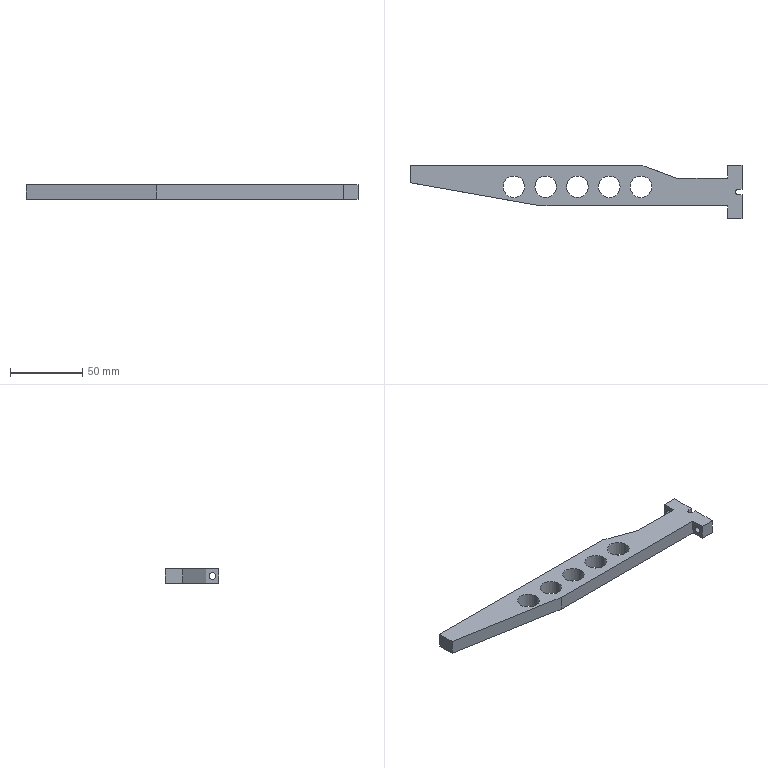Part | 1 solid | 43 faces | box 230 x 37.2 x 10 mm | volume 44801 mm3 | cylinder 21 | plane 16 | cone 6 | commonest cylinder face diameters 15 x10 2.5 x6 4.5 x4 4 x1
STEP:
#1=CARTESIAN_POINT('',(15.5,3.6,0.));
#2=VERTEX_POINT('',#1);
#3=CARTESIAN_POINT('',(30.5,3.6,0.));
#4=VERTEX_POINT('',#3);
#5=CARTESIAN_POINT('',(23.,3.6,0.));
#6=DIRECTION('',(0.,0.,-1.));
#7=DIRECTION('',(-1.,0.,0.));
#8=AXIS2_PLACEMENT_3D('',#5,#6,#7);
#9=CIRCLE('',#8,7.5);
#10=EDGE_CURVE('',#2,#4,#9,.T.);
#11=ORIENTED_EDGE('',*,*,#10,.T.);
#12=CARTESIAN_POINT('',(23.,3.6,0.));
#13=DIRECTION('',(0.,0.,-1.));
#14=DIRECTION('',(-1.,0.,0.));
#15=AXIS2_PLACEMENT_3D('',#12,#13,#14);
#16=CIRCLE('',#15,7.5);
#17=EDGE_CURVE('',#4,#2,#16,.T.);
#18=ORIENTED_EDGE('',*,*,#17,.T.);
#19=EDGE_LOOP('',(#11,#18));
#20=FACE_BOUND('',#19,.T.);
#21=CARTESIAN_POINT('',(37.5,3.6,0.));
#22=VERTEX_POINT('',#21);
#23=CARTESIAN_POINT('',(52.5,3.6,0.));
#24=VERTEX_POINT('',#23);
#25=CARTESIAN_POINT('',(45.,3.6,0.));
#26=DIRECTION('',(0.,0.,-1.));
#27=DIRECTION('',(-1.,0.,0.));
#28=AXIS2_PLACEMENT_3D('',#25,#26,#27);
#29=CIRCLE('',#28,7.5);
#30=EDGE_CURVE('',#22,#24,#29,.T.);
#31=ORIENTED_EDGE('',*,*,#30,.T.);
#32=CARTESIAN_POINT('',(45.,3.6,0.));
#33=DIRECTION('',(0.,0.,-1.));
#34=DIRECTION('',(-1.,0.,0.));
#35=AXIS2_PLACEMENT_3D('',#32,#33,#34);
#36=CIRCLE('',#35,7.5);
#37=EDGE_CURVE('',#24,#22,#36,.T.);
#38=ORIENTED_EDGE('',*,*,#37,.T.);
#39=EDGE_LOOP('',(#31,#38));
#40=FACE_BOUND('',#39,.T.);
#41=CARTESIAN_POINT('',(-50.5,3.6,0.));
#42=VERTEX_POINT('',#41);
#43=CARTESIAN_POINT('',(-35.5,3.6,0.));
#44=VERTEX_POINT('',#43);
#45=CARTESIAN_POINT('',(-43.,3.6,0.));
#46=DIRECTION('',(0.,0.,-1.));
#47=DIRECTION('',(-1.,0.,0.));
#48=AXIS2_PLACEMENT_3D('',#45,#46,#47);
#49=CIRCLE('',#48,7.5);
#50=EDGE_CURVE('',#42,#44,#49,.T.);
#51=ORIENTED_EDGE('',*,*,#50,.T.);
#52=CARTESIAN_POINT('',(-43.,3.6,0.));
#53=DIRECTION('',(0.,0.,-1.));
#54=DIRECTION('',(-1.,0.,0.));
#55=AXIS2_PLACEMENT_3D('',#52,#53,#54);
#56=CIRCLE('',#55,7.5);
#57=EDGE_CURVE('',#44,#42,#56,.T.);
#58=ORIENTED_EDGE('',*,*,#57,.T.);
#59=EDGE_LOOP('',(#51,#58));
#60=FACE_BOUND('',#59,.T.);
#61=CARTESIAN_POINT('',(-28.5,3.6,0.));
#62=VERTEX_POINT('',#61);
#63=CARTESIAN_POINT('',(-13.5,3.6,0.));
#64=VERTEX_POINT('',#63);
#65=CARTESIAN_POINT('',(-21.,3.6,0.));
#66=DIRECTION('',(0.,0.,-1.));
#67=DIRECTION('',(-1.,0.,0.));
#68=AXIS2_PLACEMENT_3D('',#65,#66,#67);
#69=CIRCLE('',#68,7.5);
#70=EDGE_CURVE('',#62,#64,#69,.T.);
#71=ORIENTED_EDGE('',*,*,#70,.T.);
#72=CARTESIAN_POINT('',(-21.,3.6,0.));
#73=DIRECTION('',(0.,0.,-1.));
#74=DIRECTION('',(-1.,0.,0.));
#75=AXIS2_PLACEMENT_3D('',#72,#73,#74);
#76=CIRCLE('',#75,7.5);
#77=EDGE_CURVE('',#64,#62,#76,.T.);
#78=ORIENTED_EDGE('',*,*,#77,.T.);
#79=EDGE_LOOP('',(#71,#78));
#80=FACE_BOUND('',#79,.T.);
#81=CARTESIAN_POINT('',(-6.5,3.6,0.));
#82=VERTEX_POINT('',#81);
#83=CARTESIAN_POINT('',(8.5,3.6,0.));
#84=VERTEX_POINT('',#83);
#85=CARTESIAN_POINT('',(1.,3.6,0.));
#86=DIRECTION('',(0.,0.,-1.));
#87=DIRECTION('',(-1.,0.,0.));
#88=AXIS2_PLACEMENT_3D('',#85,#86,#87);
#89=CIRCLE('',#88,7.5);
#90=EDGE_CURVE('',#82,#84,#89,.T.);
#91=ORIENTED_EDGE('',*,*,#90,.T.);
#92=CARTESIAN_POINT('',(1.,3.6,0.));
#93=DIRECTION('',(0.,0.,-1.));
#94=DIRECTION('',(-1.,0.,0.));
#95=AXIS2_PLACEMENT_3D('',#92,#93,#94);
#96=CIRCLE('',#95,7.5);
#97=EDGE_CURVE('',#84,#82,#96,.T.);
#98=ORIENTED_EDGE('',*,*,#97,.T.);
#99=EDGE_LOOP('',(#91,#98));
#100=FACE_BOUND('',#99,.T.);
#101=CARTESIAN_POINT('',(112.5,2.,0.));
#102=VERTEX_POINT('',#101);
#103=CARTESIAN_POINT('',(112.5,-2.,0.));
#104=VERTEX_POINT('',#103);
#105=CARTESIAN_POINT('',(112.5,0.,0.));
#106=DIRECTION('',(0.,0.,1.));
#107=DIRECTION('',(1.,0.,0.));
#108=AXIS2_PLACEMENT_3D('',#105,#106,#107);
#109=CIRCLE('',#108,2.);
#110=EDGE_CURVE('',#102,#104,#109,.T.);
#111=ORIENTED_EDGE('',*,*,#110,.F.);
#112=CARTESIAN_POINT('',(115.,2.,0.));
#113=VERTEX_POINT('',#112);
#114=CARTESIAN_POINT('',(115.,2.,0.));
#115=DIRECTION('',(1.,0.,0.));
#116=VECTOR('',#115,1000.);
#117=LINE('',#114,#116);
#118=EDGE_CURVE('',#102,#113,#117,.T.);
#119=ORIENTED_EDGE('',*,*,#118,.T.);
#120=CARTESIAN_POINT('',(115.,18.6,0.));
#121=VERTEX_POINT('',#120);
#122=CARTESIAN_POINT('',(115.,18.6,0.));
#123=DIRECTION('',(0.,-1.,0.));
#124=VECTOR('',#123,1000.);
#125=LINE('',#122,#124);
#126=EDGE_CURVE('',#121,#113,#125,.T.);
#127=ORIENTED_EDGE('',*,*,#126,.F.);
#128=CARTESIAN_POINT('',(105.,18.6,0.));
#129=VERTEX_POINT('',#128);
#130=CARTESIAN_POINT('',(115.,18.6,0.));
#131=DIRECTION('',(1.,0.,0.));
#132=VECTOR('',#131,1000.);
#133=LINE('',#130,#132);
#134=EDGE_CURVE('',#129,#121,#133,.T.);
#135=ORIENTED_EDGE('',*,*,#134,.F.);
#136=CARTESIAN_POINT('',(105.,9.6,0.));
#137=VERTEX_POINT('',#136);
#138=CARTESIAN_POINT('',(105.,18.6,0.));
#139=DIRECTION('',(0.,-1.,0.));
#140=VECTOR('',#139,1000.);
#141=LINE('',#138,#140);
#142=EDGE_CURVE('',#129,#137,#141,.T.);
#143=ORIENTED_EDGE('',*,*,#142,.T.);
#144=CARTESIAN_POINT('',(69.727,9.6,0.));
#145=VERTEX_POINT('',#144);
#146=CARTESIAN_POINT('',(105.,9.6,0.));
#147=DIRECTION('',(-1.,0.,0.));
#148=VECTOR('',#147,1000.);
#149=LINE('',#146,#148);
#150=EDGE_CURVE('',#137,#145,#149,.T.);
#151=ORIENTED_EDGE('',*,*,#150,.T.);
#152=CARTESIAN_POINT('',(45.,18.6,0.));
#153=VERTEX_POINT('',#152);
#154=CARTESIAN_POINT('',(69.727,9.6,0.));
#155=DIRECTION('',(-0.9397,0.342,0.));
#156=VECTOR('',#155,1000.);
#157=LINE('',#154,#156);
#158=EDGE_CURVE('',#145,#153,#157,.T.);
#159=ORIENTED_EDGE('',*,*,#158,.T.);
#160=CARTESIAN_POINT('',(-115.,18.6,0.));
#161=VERTEX_POINT('',#160);
#162=CARTESIAN_POINT('',(115.,18.6,0.));
#163=DIRECTION('',(1.,0.,0.));
#164=VECTOR('',#163,1000.);
#165=LINE('',#162,#164);
#166=EDGE_CURVE('',#161,#153,#165,.T.);
#167=ORIENTED_EDGE('',*,*,#166,.F.);
#168=CARTESIAN_POINT('',(-115.,6.4,0.));
#169=VERTEX_POINT('',#168);
#170=CARTESIAN_POINT('',(-115.,18.6,0.));
#171=DIRECTION('',(0.,1.,0.));
#172=VECTOR('',#171,1000.);
#173=LINE('',#170,#172);
#174=EDGE_CURVE('',#169,#161,#173,.T.);
#175=ORIENTED_EDGE('',*,*,#174,.F.);
#176=CARTESIAN_POINT('',(-24.259,-9.6,0.));
#177=VERTEX_POINT('',#176);
#178=CARTESIAN_POINT('',(-24.259,-9.6,0.));
#179=DIRECTION('',(0.9848,-0.1736,0.));
#180=VECTOR('',#179,1000.);
#181=LINE('',#178,#180);
#182=EDGE_CURVE('',#169,#177,#181,.T.);
#183=ORIENTED_EDGE('',*,*,#182,.T.);
#184=CARTESIAN_POINT('',(105.,-9.6,0.));
#185=VERTEX_POINT('',#184);
#186=CARTESIAN_POINT('',(105.,-9.6,0.));
#187=DIRECTION('',(1.,0.,0.));
#188=VECTOR('',#187,1000.);
#189=LINE('',#186,#188);
#190=EDGE_CURVE('',#177,#185,#189,.T.);
#191=ORIENTED_EDGE('',*,*,#190,.T.);
#192=CARTESIAN_POINT('',(105.,-18.6,0.));
#193=VERTEX_POINT('',#192);
#194=CARTESIAN_POINT('',(105.,-18.6,0.));
#195=DIRECTION('',(0.,-1.,0.));
#196=VECTOR('',#195,1000.);
#197=LINE('',#194,#196);
#198=EDGE_CURVE('',#185,#193,#197,.T.);
#199=ORIENTED_EDGE('',*,*,#198,.T.);
#200=CARTESIAN_POINT('',(115.,-18.6,0.));
#201=VERTEX_POINT('',#200);
#202=CARTESIAN_POINT('',(115.,-18.6,0.));
#203=DIRECTION('',(-1.,0.,0.));
#204=VECTOR('',#203,1000.);
#205=LINE('',#202,#204);
#206=EDGE_CURVE('',#201,#193,#205,.T.);
#207=ORIENTED_EDGE('',*,*,#206,.F.);
#208=CARTESIAN_POINT('',(115.,-2.,0.));
#209=VERTEX_POINT('',#208);
#210=CARTESIAN_POINT('',(115.,18.6,0.));
#211=DIRECTION('',(0.,-1.,0.));
#212=VECTOR('',#211,1000.);
#213=LINE('',#210,#212);
#214=EDGE_CURVE('',#209,#201,#213,.T.);
#215=ORIENTED_EDGE('',*,*,#214,.F.);
#216=CARTESIAN_POINT('',(115.,-2.,0.));
#217=DIRECTION('',(-1.,0.,0.));
#218=VECTOR('',#217,1000.);
#219=LINE('',#216,#218);
#220=EDGE_CURVE('',#209,#104,#219,.T.);
#221=ORIENTED_EDGE('',*,*,#220,.T.);
#222=EDGE_LOOP('',(#111,#119,#127,#135,#143,#151,#159,#167,#175,#183,#191,#199,#207,#215,#221));
#223=FACE_BOUND('',#222,.T.);
#224=CARTESIAN_POINT('',(0.,0.,0.));
#225=DIRECTION('',(0.,0.,-1.));
#226=DIRECTION('',(1.,0.,0.));
#227=AXIS2_PLACEMENT_3D('',#224,#225,#226);
#228=PLANE('',#227);
#229=ADVANCED_FACE('',(#20,#40,#60,#80,#100,#223),#228,.F.);
#230=CARTESIAN_POINT('',(115.,-16.35,-5.));
#231=VERTEX_POINT('',#230);
#232=CARTESIAN_POINT('',(115.,-11.85,-5.));
#233=VERTEX_POINT('',#232);
#234=CARTESIAN_POINT('',(115.,-14.1,-5.));
#235=DIRECTION('',(-1.,0.,0.));
#236=DIRECTION('',(0.,-1.,0.));
#237=AXIS2_PLACEMENT_3D('',#234,#235,#236);
#238=CIRCLE('',#237,2.25);
#239=EDGE_CURVE('',#231,#233,#238,.T.);
#240=ORIENTED_EDGE('',*,*,#239,.F.);
#241=CARTESIAN_POINT('',(105.,-16.35,-5.));
#242=VERTEX_POINT('',#241);
#243=CARTESIAN_POINT('',(115.,-16.35,-5.));
#244=DIRECTION('',(-1.,0.,0.));
#245=VECTOR('',#244,1000.);
#246=LINE('',#243,#245);
#247=EDGE_CURVE('',#231,#242,#246,.T.);
#248=ORIENTED_EDGE('',*,*,#247,.T.);
#249=CARTESIAN_POINT('',(105.,-11.85,-5.));
#250=VERTEX_POINT('',#249);
#251=CARTESIAN_POINT('',(105.,-14.1,-5.));
#252=DIRECTION('',(-1.,0.,0.));
#253=DIRECTION('',(0.,-1.,0.));
#254=AXIS2_PLACEMENT_3D('',#251,#252,#253);
#255=CIRCLE('',#254,2.25);
#256=EDGE_CURVE('',#242,#250,#255,.T.);
#257=ORIENTED_EDGE('',*,*,#256,.T.);
#258=CARTESIAN_POINT('',(115.,-11.85,-5.));
#259=DIRECTION('',(-1.,0.,0.));
#260=VECTOR('',#259,1000.);
#261=LINE('',#258,#260);
#262=EDGE_CURVE('',#233,#250,#261,.T.);
#263=ORIENTED_EDGE('',*,*,#262,.F.);
#264=EDGE_LOOP('',(#240,#248,#257,#263));
#265=FACE_BOUND('',#264,.T.);
#266=CARTESIAN_POINT('',(115.,-14.1,-5.));
#267=DIRECTION('',(-1.,0.,0.));
#268=DIRECTION('',(0.,-1.,0.));
#269=AXIS2_PLACEMENT_3D('',#266,#267,#268);
#270=CYLINDRICAL_SURFACE('',#269,2.25);
#271=ADVANCED_FACE('',(#265),#270,.F.);
#272=CARTESIAN_POINT('',(115.,11.85,-5.));
#273=VERTEX_POINT('',#272);
#274=CARTESIAN_POINT('',(115.,16.35,-5.));
#275=VERTEX_POINT('',#274);
#276=CARTESIAN_POINT('',(115.,14.1,-5.));
#277=DIRECTION('',(-1.,0.,0.));
#278=DIRECTION('',(0.,1.,0.));
#279=AXIS2_PLACEMENT_3D('',#276,#277,#278);
#280=CIRCLE('',#279,2.25);
#281=EDGE_CURVE('',#273,#275,#280,.T.);
#282=ORIENTED_EDGE('',*,*,#281,.F.);
#283=CARTESIAN_POINT('',(105.,11.85,-5.));
#284=VERTEX_POINT('',#283);
#285=CARTESIAN_POINT('',(115.,11.85,-5.));
#286=DIRECTION('',(-1.,0.,0.));
#287=VECTOR('',#286,1000.);
#288=LINE('',#285,#287);
#289=EDGE_CURVE('',#273,#284,#288,.T.);
#290=ORIENTED_EDGE('',*,*,#289,.T.);
#291=CARTESIAN_POINT('',(105.,16.35,-5.));
#292=VERTEX_POINT('',#291);
#293=CARTESIAN_POINT('',(105.,14.1,-5.));
#294=DIRECTION('',(-1.,0.,0.));
#295=DIRECTION('',(0.,1.,0.));
#296=AXIS2_PLACEMENT_3D('',#293,#294,#295);
#297=CIRCLE('',#296,2.25);
#298=EDGE_CURVE('',#284,#292,#297,.T.);
#299=ORIENTED_EDGE('',*,*,#298,.T.);
#300=CARTESIAN_POINT('',(115.,16.35,-5.));
#301=DIRECTION('',(-1.,0.,0.));
#302=VECTOR('',#301,1000.);
#303=LINE('',#300,#302);
#304=EDGE_CURVE('',#275,#292,#303,.T.);
#305=ORIENTED_EDGE('',*,*,#304,.F.);
#306=EDGE_LOOP('',(#282,#290,#299,#305));
#307=FACE_BOUND('',#306,.T.);
#308=CARTESIAN_POINT('',(115.,14.1,-5.));
#309=DIRECTION('',(-1.,0.,0.));
#310=DIRECTION('',(0.,-1.,0.));
#311=AXIS2_PLACEMENT_3D('',#308,#309,#310);
#312=CYLINDRICAL_SURFACE('',#311,2.25);
#313=ADVANCED_FACE('',(#307),#312,.F.);
#314=CARTESIAN_POINT('',(55.,11.1,-6.25));
#315=VERTEX_POINT('',#314);
#316=CARTESIAN_POINT('',(55.,10.349,-5.));
#317=VERTEX_POINT('',#316);
#318=CARTESIAN_POINT('',(55.,11.1,-6.25));
#319=DIRECTION('',(0.,0.515,-0.8572));
#320=VECTOR('',#319,1000.);
#321=LINE('',#318,#320);
#322=EDGE_CURVE('',#315,#317,#321,.F.);
#323=ORIENTED_EDGE('',*,*,#322,.T.);
#324=CARTESIAN_POINT('',(55.,11.1,-3.75));
#325=VERTEX_POINT('',#324);
#326=CARTESIAN_POINT('',(55.,11.1,-3.75));
#327=DIRECTION('',(0.,0.515,0.8572));
#328=VECTOR('',#327,1000.);
#329=LINE('',#326,#328);
#330=EDGE_CURVE('',#325,#317,#329,.F.);
#331=ORIENTED_EDGE('',*,*,#330,.F.);
#332=CARTESIAN_POINT('',(55.,11.1,-5.));
#333=DIRECTION('',(0.,1.,0.));
#334=DIRECTION('',(0.,0.,-1.));
#335=AXIS2_PLACEMENT_3D('',#332,#333,#334);
#336=CIRCLE('',#335,1.25);
#337=EDGE_CURVE('',#325,#315,#336,.T.);
#338=ORIENTED_EDGE('',*,*,#337,.T.);
#339=EDGE_LOOP('',(#323,#331,#338));
#340=FACE_BOUND('',#339,.T.);
#341=CARTESIAN_POINT('',(55.,11.1,-5.));
#342=DIRECTION('',(0.,1.,0.));
#343=DIRECTION('',(0.,0.,1.));
#344=AXIS2_PLACEMENT_3D('',#341,#342,#343);
#345=CONICAL_SURFACE('',#344,1.25,1.03);
#346=ADVANCED_FACE('',(#340),#345,.F.);
#347=ORIENTED_EDGE('',*,*,#337,.F.);
#348=CARTESIAN_POINT('',(55.,14.96,-3.75));
#349=VERTEX_POINT('',#348);
#350=CARTESIAN_POINT('',(55.,18.6,-3.75));
#351=DIRECTION('',(0.,1.,0.));
#352=VECTOR('',#351,1000.);
#353=LINE('',#350,#352);
#354=EDGE_CURVE('',#349,#325,#353,.F.);
#355=ORIENTED_EDGE('',*,*,#354,.F.);
#356=CARTESIAN_POINT('',(55.,14.96,-6.25));
#357=VERTEX_POINT('',#356);
#358=CARTESIAN_POINT('',(55.,14.96,-6.25));
#359=CARTESIAN_POINT('',(57.5,14.05,-6.25));
#360=CARTESIAN_POINT('',(57.5,14.05,-3.75));
#361=CARTESIAN_POINT('',(55.,14.96,-3.75));
#362=(BOUNDED_CURVE()B_SPLINE_CURVE(3,(#358,#359,#360,#361),.UNSPECIFIED.,.F.,.F.)B_SPLINE_CURVE_WITH_KNOTS((4,4),(0.,1.),.PIECEWISE_BEZIER_KNOTS.)CURVE()GEOMETRIC_REPRESENTATION_ITEM()RATIONAL_B_SPLINE_CURVE((1.,0.3333,0.3333,1.))REPRESENTATION_ITEM(''));
#363=EDGE_CURVE('',#357,#349,#362,.T.);
#364=ORIENTED_EDGE('',*,*,#363,.F.);
#365=CARTESIAN_POINT('',(55.,18.6,-6.25));
#366=DIRECTION('',(0.,1.,0.));
#367=VECTOR('',#366,1000.);
#368=LINE('',#365,#367);
#369=EDGE_CURVE('',#357,#315,#368,.F.);
#370=ORIENTED_EDGE('',*,*,#369,.T.);
#371=EDGE_LOOP('',(#347,#355,#364,#370));
#372=FACE_BOUND('',#371,.T.);
#373=CARTESIAN_POINT('',(55.,18.6,-5.));
#374=DIRECTION('',(0.,1.,0.));
#375=DIRECTION('',(0.,0.,1.));
#376=AXIS2_PLACEMENT_3D('',#373,#374,#375);
#377=CYLINDRICAL_SURFACE('',#376,1.25);
#378=ADVANCED_FACE('',(#372),#377,.F.);
#379=CARTESIAN_POINT('',(-25.,11.1,-3.75));
#380=VERTEX_POINT('',#379);
#381=CARTESIAN_POINT('',(-25.,11.1,-6.25));
#382=VERTEX_POINT('',#381);
#383=CARTESIAN_POINT('',(-25.,11.1,-5.));
#384=DIRECTION('',(0.,1.,0.));
#385=DIRECTION('',(0.,0.,-1.));
#386=AXIS2_PLACEMENT_3D('',#383,#384,#385);
#387=CIRCLE('',#386,1.25);
#388=EDGE_CURVE('',#380,#382,#387,.T.);
#389=ORIENTED_EDGE('',*,*,#388,.F.);
#390=CARTESIAN_POINT('',(-25.,18.6,-3.75));
#391=VERTEX_POINT('',#390);
#392=CARTESIAN_POINT('',(-25.,18.6,-3.75));
#393=DIRECTION('',(0.,1.,0.));
#394=VECTOR('',#393,1000.);
#395=LINE('',#392,#394);
#396=EDGE_CURVE('',#391,#380,#395,.F.);
#397=ORIENTED_EDGE('',*,*,#396,.F.);
#398=CARTESIAN_POINT('',(-25.,18.6,-6.25));
#399=VERTEX_POINT('',#398);
#400=CARTESIAN_POINT('',(-25.,18.6,-5.));
#401=DIRECTION('',(0.,1.,0.));
#402=DIRECTION('',(0.,0.,-1.));
#403=AXIS2_PLACEMENT_3D('',#400,#401,#402);
#404=CIRCLE('',#403,1.25);
#405=EDGE_CURVE('',#391,#399,#404,.T.);
#406=ORIENTED_EDGE('',*,*,#405,.T.);
#407=CARTESIAN_POINT('',(-25.,18.6,-6.25));
#408=DIRECTION('',(0.,1.,0.));
#409=VECTOR('',#408,1000.);
#410=LINE('',#407,#409);
#411=EDGE_CURVE('',#399,#382,#410,.F.);
#412=ORIENTED_EDGE('',*,*,#411,.T.);
#413=EDGE_LOOP('',(#389,#397,#406,#412));
#414=FACE_BOUND('',#413,.T.);
#415=CARTESIAN_POINT('',(-25.,18.6,-5.));
#416=DIRECTION('',(0.,1.,0.));
#417=DIRECTION('',(0.,0.,1.));
#418=AXIS2_PLACEMENT_3D('',#415,#416,#417);
#419=CYLINDRICAL_SURFACE('',#418,1.25);
#420=ADVANCED_FACE('',(#414),#419,.F.);
#421=CARTESIAN_POINT('',(-25.,10.349,-5.));
#422=VERTEX_POINT('',#421);
#423=CARTESIAN_POINT('',(-25.,11.1,-6.25));
#424=DIRECTION('',(0.,0.515,-0.8572));
#425=VECTOR('',#424,1000.);
#426=LINE('',#423,#425);
#427=EDGE_CURVE('',#382,#422,#426,.F.);
#428=ORIENTED_EDGE('',*,*,#427,.T.);
#429=CARTESIAN_POINT('',(-25.,11.1,-3.75));
#430=DIRECTION('',(0.,0.515,0.8572));
#431=VECTOR('',#430,1000.);
#432=LINE('',#429,#431);
#433=EDGE_CURVE('',#380,#422,#432,.F.);
#434=ORIENTED_EDGE('',*,*,#433,.F.);
#435=ORIENTED_EDGE('',*,*,#388,.T.);
#436=EDGE_LOOP('',(#428,#434,#435));
#437=FACE_BOUND('',#436,.T.);
#438=CARTESIAN_POINT('',(-25.,11.1,-5.));
#439=DIRECTION('',(0.,1.,0.));
#440=DIRECTION('',(0.,0.,1.));
#441=AXIS2_PLACEMENT_3D('',#438,#439,#440);
#442=CONICAL_SURFACE('',#441,1.25,1.03);
#443=ADVANCED_FACE('',(#437),#442,.F.);
#444=CARTESIAN_POINT('',(-105.,11.1,-3.75));
#445=VERTEX_POINT('',#444);
#446=CARTESIAN_POINT('',(-105.,11.1,-6.25));
#447=VERTEX_POINT('',#446);
#448=CARTESIAN_POINT('',(-105.,11.1,-5.));
#449=DIRECTION('',(0.,1.,0.));
#450=DIRECTION('',(0.,0.,-1.));
#451=AXIS2_PLACEMENT_3D('',#448,#449,#450);
#452=CIRCLE('',#451,1.25);
#453=EDGE_CURVE('',#445,#447,#452,.T.);
#454=ORIENTED_EDGE('',*,*,#453,.F.);
#455=CARTESIAN_POINT('',(-105.,18.6,-3.75));
#456=VERTEX_POINT('',#455);
#457=CARTESIAN_POINT('',(-105.,18.6,-3.75));
#458=DIRECTION('',(0.,1.,0.));
#459=VECTOR('',#458,1000.);
#460=LINE('',#457,#459);
#461=EDGE_CURVE('',#456,#445,#460,.F.);
#462=ORIENTED_EDGE('',*,*,#461,.F.);
#463=CARTESIAN_POINT('',(-105.,18.6,-6.25));
#464=VERTEX_POINT('',#463);
#465=CARTESIAN_POINT('',(-105.,18.6,-5.));
#466=DIRECTION('',(0.,1.,0.));
#467=DIRECTION('',(0.,0.,-1.));
#468=AXIS2_PLACEMENT_3D('',#465,#466,#467);
#469=CIRCLE('',#468,1.25);
#470=EDGE_CURVE('',#456,#464,#469,.T.);
#471=ORIENTED_EDGE('',*,*,#470,.T.);
#472=CARTESIAN_POINT('',(-105.,18.6,-6.25));
#473=DIRECTION('',(0.,1.,0.));
#474=VECTOR('',#473,1000.);
#475=LINE('',#472,#474);
#476=EDGE_CURVE('',#464,#447,#475,.F.);
#477=ORIENTED_EDGE('',*,*,#476,.T.);
#478=EDGE_LOOP('',(#454,#462,#471,#477));
#479=FACE_BOUND('',#478,.T.);
#480=CARTESIAN_POINT('',(-105.,18.6,-5.));
#481=DIRECTION('',(0.,1.,0.));
#482=DIRECTION('',(0.,0.,1.));
#483=AXIS2_PLACEMENT_3D('',#480,#481,#482);
#484=CYLINDRICAL_SURFACE('',#483,1.25);
#485=ADVANCED_FACE('',(#479),#484,.F.);
#486=CARTESIAN_POINT('',(-105.,10.349,-5.));
#487=VERTEX_POINT('',#486);
#488=CARTESIAN_POINT('',(-105.,11.1,-6.25));
#489=DIRECTION('',(0.,0.515,-0.8572));
#490=VECTOR('',#489,1000.);
#491=LINE('',#488,#490);
#492=EDGE_CURVE('',#447,#487,#491,.F.);
#493=ORIENTED_EDGE('',*,*,#492,.T.);
#494=CARTESIAN_POINT('',(-105.,11.1,-3.75));
#495=DIRECTION('',(0.,0.515,0.8572));
#496=VECTOR('',#495,1000.);
#497=LINE('',#494,#496);
#498=EDGE_CURVE('',#445,#487,#497,.F.);
#499=ORIENTED_EDGE('',*,*,#498,.F.);
#500=ORIENTED_EDGE('',*,*,#453,.T.);
#501=EDGE_LOOP('',(#493,#499,#500));
#502=FACE_BOUND('',#501,.T.);
#503=CARTESIAN_POINT('',(-105.,11.1,-5.));
#504=DIRECTION('',(0.,1.,0.));
#505=DIRECTION('',(0.,0.,1.));
#506=AXIS2_PLACEMENT_3D('',#503,#504,#505);
#507=CONICAL_SURFACE('',#506,1.25,1.03);
#508=ADVANCED_FACE('',(#502),#507,.F.);
#509=ORIENTED_EDGE('',*,*,#97,.F.);
#510=CARTESIAN_POINT('',(8.5,3.6,-10.));
#511=VERTEX_POINT('',#510);
#512=CARTESIAN_POINT('',(8.5,3.6,0.));
#513=DIRECTION('',(0.,0.,-1.));
#514=VECTOR('',#513,1000.);
#515=LINE('',#512,#514);
#516=EDGE_CURVE('',#511,#84,#515,.F.);
#517=ORIENTED_EDGE('',*,*,#516,.F.);
#518=CARTESIAN_POINT('',(-6.5,3.6,-10.));
#519=VERTEX_POINT('',#518);
#520=CARTESIAN_POINT('',(1.,3.6,-10.));
#521=DIRECTION('',(0.,0.,-1.));
#522=DIRECTION('',(-1.,0.,0.));
#523=AXIS2_PLACEMENT_3D('',#520,#521,#522);
#524=CIRCLE('',#523,7.5);
#525=EDGE_CURVE('',#511,#519,#524,.T.);
#526=ORIENTED_EDGE('',*,*,#525,.T.);
#527=CARTESIAN_POINT('',(-6.5,3.6,0.));
#528=DIRECTION('',(0.,0.,-1.));
#529=VECTOR('',#528,1000.);
#530=LINE('',#527,#529);
#531=EDGE_CURVE('',#519,#82,#530,.F.);
#532=ORIENTED_EDGE('',*,*,#531,.T.);
#533=EDGE_LOOP('',(#509,#517,#526,#532));
#534=FACE_BOUND('',#533,.T.);
#535=CARTESIAN_POINT('',(1.,3.6,0.));
#536=DIRECTION('',(0.,0.,-1.));
#537=DIRECTION('',(1.,0.,0.));
#538=AXIS2_PLACEMENT_3D('',#535,#536,#537);
#539=CYLINDRICAL_SURFACE('',#538,7.5);
#540=ADVANCED_FACE('',(#534),#539,.F.);
#541=ORIENTED_EDGE('',*,*,#77,.F.);
#542=CARTESIAN_POINT('',(-13.5,3.6,-10.));
#543=VERTEX_POINT('',#542);
#544=CARTESIAN_POINT('',(-13.5,3.6,0.));
#545=DIRECTION('',(0.,0.,-1.));
#546=VECTOR('',#545,1000.);
#547=LINE('',#544,#546);
#548=EDGE_CURVE('',#543,#64,#547,.F.);
#549=ORIENTED_EDGE('',*,*,#548,.F.);
#550=CARTESIAN_POINT('',(-28.5,3.6,-10.));
#551=VERTEX_POINT('',#550);
#552=CARTESIAN_POINT('',(-21.,3.6,-10.));
#553=DIRECTION('',(0.,0.,-1.));
#554=DIRECTION('',(-1.,0.,0.));
#555=AXIS2_PLACEMENT_3D('',#552,#553,#554);
#556=CIRCLE('',#555,7.5);
#557=EDGE_CURVE('',#543,#551,#556,.T.);
#558=ORIENTED_EDGE('',*,*,#557,.T.);
#559=CARTESIAN_POINT('',(-28.5,3.6,0.));
#560=DIRECTION('',(0.,0.,-1.));
#561=VECTOR('',#560,1000.);
#562=LINE('',#559,#561);
#563=EDGE_CURVE('',#551,#62,#562,.F.);
#564=ORIENTED_EDGE('',*,*,#563,.T.);
#565=EDGE_LOOP('',(#541,#549,#558,#564));
#566=FACE_BOUND('',#565,.T.);
#567=CARTESIAN_POINT('',(-21.,3.6,0.));
#568=DIRECTION('',(0.,0.,-1.));
#569=DIRECTION('',(1.,0.,0.));
#570=AXIS2_PLACEMENT_3D('',#567,#568,#569);
#571=CYLINDRICAL_SURFACE('',#570,7.5);
#572=ADVANCED_FACE('',(#566),#571,.F.);
#573=ORIENTED_EDGE('',*,*,#57,.F.);
#574=CARTESIAN_POINT('',(-35.5,3.6,-10.));
#575=VERTEX_POINT('',#574);
#576=CARTESIAN_POINT('',(-35.5,3.6,0.));
#577=DIRECTION('',(0.,0.,-1.));
#578=VECTOR('',#577,1000.);
#579=LINE('',#576,#578);
#580=EDGE_CURVE('',#575,#44,#579,.F.);
#581=ORIENTED_EDGE('',*,*,#580,.F.);
#582=CARTESIAN_POINT('',(-50.5,3.6,-10.));
#583=VERTEX_POINT('',#582);
#584=CARTESIAN_POINT('',(-43.,3.6,-10.));
#585=DIRECTION('',(0.,0.,-1.));
#586=DIRECTION('',(-1.,0.,0.));
#587=AXIS2_PLACEMENT_3D('',#584,#585,#586);
#588=CIRCLE('',#587,7.5);
#589=EDGE_CURVE('',#575,#583,#588,.T.);
#590=ORIENTED_EDGE('',*,*,#589,.T.);
#591=CARTESIAN_POINT('',(-50.5,3.6,0.));
#592=DIRECTION('',(0.,0.,-1.));
#593=VECTOR('',#592,1000.);
#594=LINE('',#591,#593);
#595=EDGE_CURVE('',#583,#42,#594,.F.);
#596=ORIENTED_EDGE('',*,*,#595,.T.);
#597=EDGE_LOOP('',(#573,#581,#590,#596));
#598=FACE_BOUND('',#597,.T.);
#599=CARTESIAN_POINT('',(-43.,3.6,0.));
#600=DIRECTION('',(0.,0.,-1.));
#601=DIRECTION('',(1.,0.,0.));
#602=AXIS2_PLACEMENT_3D('',#599,#600,#601);
#603=CYLINDRICAL_SURFACE('',#602,7.5);
#604=ADVANCED_FACE('',(#598),#603,.F.);
#605=ORIENTED_EDGE('',*,*,#37,.F.);
#606=CARTESIAN_POINT('',(52.5,3.6,-10.));
#607=VERTEX_POINT('',#606);
#608=CARTESIAN_POINT('',(52.5,3.6,0.));
#609=DIRECTION('',(0.,0.,-1.));
#610=VECTOR('',#609,1000.);
#611=LINE('',#608,#610);
#612=EDGE_CURVE('',#607,#24,#611,.F.);
#613=ORIENTED_EDGE('',*,*,#612,.F.);
#614=CARTESIAN_POINT('',(37.5,3.6,-10.));
#615=VERTEX_POINT('',#614);
#616=CARTESIAN_POINT('',(45.,3.6,-10.));
#617=DIRECTION('',(0.,0.,-1.));
#618=DIRECTION('',(-1.,0.,0.));
#619=AXIS2_PLACEMENT_3D('',#616,#617,#618);
#620=CIRCLE('',#619,7.5);
#621=EDGE_CURVE('',#607,#615,#620,.T.);
#622=ORIENTED_EDGE('',*,*,#621,.T.);
#623=CARTESIAN_POINT('',(37.5,3.6,0.));
#624=DIRECTION('',(0.,0.,-1.));
#625=VECTOR('',#624,1000.);
#626=LINE('',#623,#625);
#627=EDGE_CURVE('',#615,#22,#626,.F.);
#628=ORIENTED_EDGE('',*,*,#627,.T.);
#629=EDGE_LOOP('',(#605,#613,#622,#628));
#630=FACE_BOUND('',#629,.T.);
#631=CARTESIAN_POINT('',(45.,3.6,0.));
#632=DIRECTION('',(0.,0.,-1.));
#633=DIRECTION('',(1.,0.,0.));
#634=AXIS2_PLACEMENT_3D('',#631,#632,#633);
#635=CYLINDRICAL_SURFACE('',#634,7.5);
#636=ADVANCED_FACE('',(#630),#635,.F.);
#637=ORIENTED_EDGE('',*,*,#17,.F.);
#638=CARTESIAN_POINT('',(30.5,3.6,-10.));
#639=VERTEX_POINT('',#638);
#640=CARTESIAN_POINT('',(30.5,3.6,0.));
#641=DIRECTION('',(0.,0.,-1.));
#642=VECTOR('',#641,1000.);
#643=LINE('',#640,#642);
#644=EDGE_CURVE('',#639,#4,#643,.F.);
#645=ORIENTED_EDGE('',*,*,#644,.F.);
#646=CARTESIAN_POINT('',(15.5,3.6,-10.));
#647=VERTEX_POINT('',#646);
#648=CARTESIAN_POINT('',(23.,3.6,-10.));
#649=DIRECTION('',(0.,0.,-1.));
#650=DIRECTION('',(-1.,0.,0.));
#651=AXIS2_PLACEMENT_3D('',#648,#649,#650);
#652=CIRCLE('',#651,7.5);
#653=EDGE_CURVE('',#639,#647,#652,.T.);
#654=ORIENTED_EDGE('',*,*,#653,.T.);
#655=CARTESIAN_POINT('',(15.5,3.6,0.));
#656=DIRECTION('',(0.,0.,-1.));
#657=VECTOR('',#656,1000.);
#658=LINE('',#655,#657);
#659=EDGE_CURVE('',#647,#2,#658,.F.);
#660=ORIENTED_EDGE('',*,*,#659,.T.);
#661=EDGE_LOOP('',(#637,#645,#654,#660));
#662=FACE_BOUND('',#661,.T.);
#663=CARTESIAN_POINT('',(23.,3.6,0.));
#664=DIRECTION('',(0.,0.,-1.));
#665=DIRECTION('',(1.,0.,0.));
#666=AXIS2_PLACEMENT_3D('',#663,#664,#665);
#667=CYLINDRICAL_SURFACE('',#666,7.5);
#668=ADVANCED_FACE('',(#662),#667,.F.);
#669=CARTESIAN_POINT('',(115.,14.1,-5.));
#670=DIRECTION('',(-1.,0.,0.));
#671=DIRECTION('',(0.,1.,0.));
#672=AXIS2_PLACEMENT_3D('',#669,#670,#671);
#673=CIRCLE('',#672,2.25);
#674=EDGE_CURVE('',#275,#273,#673,.T.);
#675=ORIENTED_EDGE('',*,*,#674,.T.);
#676=ORIENTED_EDGE('',*,*,#281,.T.);
#677=EDGE_LOOP('',(#675,#676));
#678=FACE_BOUND('',#677,.T.);
#679=ORIENTED_EDGE('',*,*,#126,.T.);
#680=CARTESIAN_POINT('',(115.,2.,-10.));
#681=VERTEX_POINT('',#680);
#682=CARTESIAN_POINT('',(115.,2.,0.));
#683=DIRECTION('',(0.,0.,-1.));
#684=VECTOR('',#683,1000.);
#685=LINE('',#682,#684);
#686=EDGE_CURVE('',#113,#681,#685,.T.);
#687=ORIENTED_EDGE('',*,*,#686,.T.);
#688=CARTESIAN_POINT('',(115.,18.6,-10.));
#689=VERTEX_POINT('',#688);
#690=CARTESIAN_POINT('',(115.,18.6,-10.));
#691=DIRECTION('',(0.,-1.,0.));
#692=VECTOR('',#691,1000.);
#693=LINE('',#690,#692);
#694=EDGE_CURVE('',#689,#681,#693,.T.);
#695=ORIENTED_EDGE('',*,*,#694,.F.);
#696=CARTESIAN_POINT('',(115.,18.6,-10.));
#697=DIRECTION('',(0.,0.,1.));
#698=VECTOR('',#697,1000.);
#699=LINE('',#696,#698);
#700=EDGE_CURVE('',#689,#121,#699,.T.);
#701=ORIENTED_EDGE('',*,*,#700,.T.);
#702=EDGE_LOOP('',(#679,#687,#695,#701));
#703=FACE_BOUND('',#702,.T.);
#704=CARTESIAN_POINT('',(115.,18.6,-10.));
#705=DIRECTION('',(-1.,0.,0.));
#706=DIRECTION('',(0.,0.,-1.));
#707=AXIS2_PLACEMENT_3D('',#704,#705,#706);
#708=PLANE('',#707);
#709=ADVANCED_FACE('',(#678,#703),#708,.F.);
#710=CARTESIAN_POINT('',(-25.,18.6,-5.));
#711=DIRECTION('',(0.,1.,0.));
#712=DIRECTION('',(0.,0.,-1.));
#713=AXIS2_PLACEMENT_3D('',#710,#711,#712);
#714=CIRCLE('',#713,1.25);
#715=EDGE_CURVE('',#399,#391,#714,.T.);
#716=ORIENTED_EDGE('',*,*,#715,.F.);
#717=ORIENTED_EDGE('',*,*,#405,.F.);
#718=EDGE_LOOP('',(#716,#717));
#719=FACE_BOUND('',#718,.T.);
#720=CARTESIAN_POINT('',(-105.,18.6,-5.));
#721=DIRECTION('',(0.,1.,0.));
#722=DIRECTION('',(0.,0.,-1.));
#723=AXIS2_PLACEMENT_3D('',#720,#721,#722);
#724=CIRCLE('',#723,1.25);
#725=EDGE_CURVE('',#464,#456,#724,.T.);
#726=ORIENTED_EDGE('',*,*,#725,.F.);
#727=ORIENTED_EDGE('',*,*,#470,.F.);
#728=EDGE_LOOP('',(#726,#727));
#729=FACE_BOUND('',#728,.T.);
#730=ORIENTED_EDGE('',*,*,#166,.T.);
#731=CARTESIAN_POINT('',(45.,18.6,-10.));
#732=VERTEX_POINT('',#731);
#733=CARTESIAN_POINT('',(45.,18.6,0.));
#734=DIRECTION('',(0.,0.,-1.));
#735=VECTOR('',#734,1000.);
#736=LINE('',#733,#735);
#737=EDGE_CURVE('',#153,#732,#736,.T.);
#738=ORIENTED_EDGE('',*,*,#737,.T.);
#739=CARTESIAN_POINT('',(-115.,18.6,-10.));
#740=VERTEX_POINT('',#739);
#741=CARTESIAN_POINT('',(115.,18.6,-10.));
#742=DIRECTION('',(1.,0.,0.));
#743=VECTOR('',#742,1000.);
#744=LINE('',#741,#743);
#745=EDGE_CURVE('',#740,#732,#744,.T.);
#746=ORIENTED_EDGE('',*,*,#745,.F.);
#747=CARTESIAN_POINT('',(-115.,18.6,-10.));
#748=DIRECTION('',(0.,0.,1.));
#749=VECTOR('',#748,1000.);
#750=LINE('',#747,#749);
#751=EDGE_CURVE('',#740,#161,#750,.T.);
#752=ORIENTED_EDGE('',*,*,#751,.T.);
#753=EDGE_LOOP('',(#730,#738,#746,#752));
#754=FACE_BOUND('',#753,.T.);
#755=CARTESIAN_POINT('',(115.,18.6,-10.));
#756=DIRECTION('',(0.,-1.,0.));
#757=DIRECTION('',(0.,0.,-1.));
#758=AXIS2_PLACEMENT_3D('',#755,#756,#757);
#759=PLANE('',#758);
#760=ADVANCED_FACE('',(#719,#729,#754),#759,.F.);
#761=CARTESIAN_POINT('',(115.,-14.1,-5.));
#762=DIRECTION('',(-1.,0.,0.));
#763=DIRECTION('',(0.,-1.,0.));
#764=AXIS2_PLACEMENT_3D('',#761,#762,#763);
#765=CIRCLE('',#764,2.25);
#766=EDGE_CURVE('',#233,#231,#765,.T.);
#767=ORIENTED_EDGE('',*,*,#766,.T.);
#768=ORIENTED_EDGE('',*,*,#239,.T.);
#769=EDGE_LOOP('',(#767,#768));
#770=FACE_BOUND('',#769,.T.);
#771=CARTESIAN_POINT('',(115.,-2.,-10.));
#772=VERTEX_POINT('',#771);
#773=CARTESIAN_POINT('',(115.,-18.6,-10.));
#774=VERTEX_POINT('',#773);
#775=CARTESIAN_POINT('',(115.,18.6,-10.));
#776=DIRECTION('',(0.,-1.,0.));
#777=VECTOR('',#776,1000.);
#778=LINE('',#775,#777);
#779=EDGE_CURVE('',#772,#774,#778,.T.);
#780=ORIENTED_EDGE('',*,*,#779,.F.);
#781=CARTESIAN_POINT('',(115.,-2.,0.));
#782=DIRECTION('',(0.,0.,-1.));
#783=VECTOR('',#782,1000.);
#784=LINE('',#781,#783);
#785=EDGE_CURVE('',#209,#772,#784,.T.);
#786=ORIENTED_EDGE('',*,*,#785,.F.);
#787=ORIENTED_EDGE('',*,*,#214,.T.);
#788=CARTESIAN_POINT('',(115.,-18.6,-10.));
#789=DIRECTION('',(0.,0.,1.));
#790=VECTOR('',#789,1000.);
#791=LINE('',#788,#790);
#792=EDGE_CURVE('',#774,#201,#791,.T.);
#793=ORIENTED_EDGE('',*,*,#792,.F.);
#794=EDGE_LOOP('',(#780,#786,#787,#793));
#795=FACE_BOUND('',#794,.T.);
#796=CARTESIAN_POINT('',(115.,18.6,-10.));
#797=DIRECTION('',(-1.,0.,0.));
#798=DIRECTION('',(0.,0.,-1.));
#799=AXIS2_PLACEMENT_3D('',#796,#797,#798);
#800=PLANE('',#799);
#801=ADVANCED_FACE('',(#770,#795),#800,.F.);
#802=ORIENTED_EDGE('',*,*,#206,.T.);
#803=CARTESIAN_POINT('',(105.,-18.6,-10.));
#804=VERTEX_POINT('',#803);
#805=CARTESIAN_POINT('',(105.,-18.6,0.));
#806=DIRECTION('',(0.,0.,-1.));
#807=VECTOR('',#806,1000.);
#808=LINE('',#805,#807);
#809=EDGE_CURVE('',#193,#804,#808,.T.);
#810=ORIENTED_EDGE('',*,*,#809,.T.);
#811=CARTESIAN_POINT('',(115.,-18.6,-10.));
#812=DIRECTION('',(-1.,0.,0.));
#813=VECTOR('',#812,1000.);
#814=LINE('',#811,#813);
#815=EDGE_CURVE('',#774,#804,#814,.T.);
#816=ORIENTED_EDGE('',*,*,#815,.F.);
#817=ORIENTED_EDGE('',*,*,#792,.T.);
#818=EDGE_LOOP('',(#802,#810,#816,#817));
#819=FACE_BOUND('',#818,.T.);
#820=CARTESIAN_POINT('',(115.,-18.6,-10.));
#821=DIRECTION('',(0.,1.,0.));
#822=DIRECTION('',(-1.,0.,0.));
#823=AXIS2_PLACEMENT_3D('',#820,#821,#822);
#824=PLANE('',#823);
#825=ADVANCED_FACE('',(#819),#824,.F.);
#826=CARTESIAN_POINT('',(-115.,6.4,-10.));
#827=VERTEX_POINT('',#826);
#828=CARTESIAN_POINT('',(-115.,18.6,-10.));
#829=DIRECTION('',(0.,1.,0.));
#830=VECTOR('',#829,1000.);
#831=LINE('',#828,#830);
#832=EDGE_CURVE('',#827,#740,#831,.T.);
#833=ORIENTED_EDGE('',*,*,#832,.F.);
#834=CARTESIAN_POINT('',(-115.,6.4,0.));
#835=DIRECTION('',(0.,0.,-1.));
#836=VECTOR('',#835,1000.);
#837=LINE('',#834,#836);
#838=EDGE_CURVE('',#169,#827,#837,.T.);
#839=ORIENTED_EDGE('',*,*,#838,.F.);
#840=ORIENTED_EDGE('',*,*,#174,.T.);
#841=ORIENTED_EDGE('',*,*,#751,.F.);
#842=EDGE_LOOP('',(#833,#839,#840,#841));
#843=FACE_BOUND('',#842,.T.);
#844=CARTESIAN_POINT('',(-115.,18.6,-10.));
#845=DIRECTION('',(1.,0.,0.));
#846=DIRECTION('',(0.,0.,1.));
#847=AXIS2_PLACEMENT_3D('',#844,#845,#846);
#848=PLANE('',#847);
#849=ADVANCED_FACE('',(#843),#848,.F.);
#850=CARTESIAN_POINT('',(105.,18.6,-10.));
#851=VERTEX_POINT('',#850);
#852=CARTESIAN_POINT('',(115.,18.6,-10.));
#853=DIRECTION('',(1.,0.,0.));
#854=VECTOR('',#853,1000.);
#855=LINE('',#852,#854);
#856=EDGE_CURVE('',#851,#689,#855,.T.);
#857=ORIENTED_EDGE('',*,*,#856,.F.);
#858=CARTESIAN_POINT('',(105.,18.6,0.));
#859=DIRECTION('',(0.,0.,-1.));
#860=VECTOR('',#859,1000.);
#861=LINE('',#858,#860);
#862=EDGE_CURVE('',#129,#851,#861,.T.);
#863=ORIENTED_EDGE('',*,*,#862,.F.);
#864=ORIENTED_EDGE('',*,*,#134,.T.);
#865=ORIENTED_EDGE('',*,*,#700,.F.);
#866=EDGE_LOOP('',(#857,#863,#864,#865));
#867=FACE_BOUND('',#866,.T.);
#868=CARTESIAN_POINT('',(115.,18.6,-10.));
#869=DIRECTION('',(0.,-1.,0.));
#870=DIRECTION('',(0.,0.,-1.));
#871=AXIS2_PLACEMENT_3D('',#868,#869,#870);
#872=PLANE('',#871);
#873=ADVANCED_FACE('',(#867),#872,.F.);
#874=CARTESIAN_POINT('',(112.5,-2.,-10.));
#875=VERTEX_POINT('',#874);
#876=CARTESIAN_POINT('',(112.5,2.,-10.));
#877=VERTEX_POINT('',#876);
#878=CARTESIAN_POINT('',(112.5,0.,-10.));
#879=DIRECTION('',(0.,0.,-1.));
#880=DIRECTION('',(-1.,0.,0.));
#881=AXIS2_PLACEMENT_3D('',#878,#879,#880);
#882=CIRCLE('',#881,2.);
#883=EDGE_CURVE('',#875,#877,#882,.T.);
#884=ORIENTED_EDGE('',*,*,#883,.F.);
#885=CARTESIAN_POINT('',(115.,-2.,-10.));
#886=DIRECTION('',(-1.,0.,0.));
#887=VECTOR('',#886,1000.);
#888=LINE('',#885,#887);
#889=EDGE_CURVE('',#772,#875,#888,.T.);
#890=ORIENTED_EDGE('',*,*,#889,.F.);
#891=ORIENTED_EDGE('',*,*,#779,.T.);
#892=ORIENTED_EDGE('',*,*,#815,.T.);
#893=CARTESIAN_POINT('',(105.,-9.6,-10.));
#894=VERTEX_POINT('',#893);
#895=CARTESIAN_POINT('',(105.,-18.6,-10.));
#896=DIRECTION('',(0.,-1.,0.));
#897=VECTOR('',#896,1000.);
#898=LINE('',#895,#897);
#899=EDGE_CURVE('',#894,#804,#898,.T.);
#900=ORIENTED_EDGE('',*,*,#899,.F.);
#901=CARTESIAN_POINT('',(-24.259,-9.6,-10.));
#902=VERTEX_POINT('',#901);
#903=CARTESIAN_POINT('',(105.,-9.6,-10.));
#904=DIRECTION('',(1.,0.,0.));
#905=VECTOR('',#904,1000.);
#906=LINE('',#903,#905);
#907=EDGE_CURVE('',#902,#894,#906,.T.);
#908=ORIENTED_EDGE('',*,*,#907,.F.);
#909=CARTESIAN_POINT('',(-24.259,-9.6,-10.));
#910=DIRECTION('',(0.9848,-0.1736,0.));
#911=VECTOR('',#910,1000.);
#912=LINE('',#909,#911);
#913=EDGE_CURVE('',#827,#902,#912,.T.);
#914=ORIENTED_EDGE('',*,*,#913,.F.);
#915=ORIENTED_EDGE('',*,*,#832,.T.);
#916=ORIENTED_EDGE('',*,*,#745,.T.);
#917=CARTESIAN_POINT('',(69.727,9.6,-10.));
#918=VERTEX_POINT('',#917);
#919=CARTESIAN_POINT('',(69.727,9.6,-10.));
#920=DIRECTION('',(-0.9397,0.342,0.));
#921=VECTOR('',#920,1000.);
#922=LINE('',#919,#921);
#923=EDGE_CURVE('',#918,#732,#922,.T.);
#924=ORIENTED_EDGE('',*,*,#923,.F.);
#925=CARTESIAN_POINT('',(105.,9.6,-10.));
#926=VERTEX_POINT('',#925);
#927=CARTESIAN_POINT('',(105.,9.6,-10.));
#928=DIRECTION('',(-1.,0.,0.));
#929=VECTOR('',#928,1000.);
#930=LINE('',#927,#929);
#931=EDGE_CURVE('',#926,#918,#930,.T.);
#932=ORIENTED_EDGE('',*,*,#931,.F.);
#933=CARTESIAN_POINT('',(105.,18.6,-10.));
#934=DIRECTION('',(0.,-1.,0.));
#935=VECTOR('',#934,1000.);
#936=LINE('',#933,#935);
#937=EDGE_CURVE('',#851,#926,#936,.T.);
#938=ORIENTED_EDGE('',*,*,#937,.F.);
#939=ORIENTED_EDGE('',*,*,#856,.T.);
#940=ORIENTED_EDGE('',*,*,#694,.T.);
#941=CARTESIAN_POINT('',(115.,2.,-10.));
#942=DIRECTION('',(1.,0.,0.));
#943=VECTOR('',#942,1000.);
#944=LINE('',#941,#943);
#945=EDGE_CURVE('',#877,#681,#944,.T.);
#946=ORIENTED_EDGE('',*,*,#945,.F.);
#947=EDGE_LOOP('',(#884,#890,#891,#892,#900,#908,#914,#915,#916,#924,#932,#938,#939,#940,#946));
#948=FACE_BOUND('',#947,.T.);
#949=CARTESIAN_POINT('',(1.,3.6,-10.));
#950=DIRECTION('',(0.,0.,-1.));
#951=DIRECTION('',(-1.,0.,0.));
#952=AXIS2_PLACEMENT_3D('',#949,#950,#951);
#953=CIRCLE('',#952,7.5);
#954=EDGE_CURVE('',#519,#511,#953,.T.);
#955=ORIENTED_EDGE('',*,*,#954,.F.);
#956=ORIENTED_EDGE('',*,*,#525,.F.);
#957=EDGE_LOOP('',(#955,#956));
#958=FACE_BOUND('',#957,.T.);
#959=CARTESIAN_POINT('',(-21.,3.6,-10.));
#960=DIRECTION('',(0.,0.,-1.));
#961=DIRECTION('',(-1.,0.,0.));
#962=AXIS2_PLACEMENT_3D('',#959,#960,#961);
#963=CIRCLE('',#962,7.5);
#964=EDGE_CURVE('',#551,#543,#963,.T.);
#965=ORIENTED_EDGE('',*,*,#964,.F.);
#966=ORIENTED_EDGE('',*,*,#557,.F.);
#967=EDGE_LOOP('',(#965,#966));
#968=FACE_BOUND('',#967,.T.);
#969=CARTESIAN_POINT('',(-43.,3.6,-10.));
#970=DIRECTION('',(0.,0.,-1.));
#971=DIRECTION('',(-1.,0.,0.));
#972=AXIS2_PLACEMENT_3D('',#969,#970,#971);
#973=CIRCLE('',#972,7.5);
#974=EDGE_CURVE('',#583,#575,#973,.T.);
#975=ORIENTED_EDGE('',*,*,#974,.F.);
#976=ORIENTED_EDGE('',*,*,#589,.F.);
#977=EDGE_LOOP('',(#975,#976));
#978=FACE_BOUND('',#977,.T.);
#979=CARTESIAN_POINT('',(45.,3.6,-10.));
#980=DIRECTION('',(0.,0.,-1.));
#981=DIRECTION('',(-1.,0.,0.));
#982=AXIS2_PLACEMENT_3D('',#979,#980,#981);
#983=CIRCLE('',#982,7.5);
#984=EDGE_CURVE('',#615,#607,#983,.T.);
#985=ORIENTED_EDGE('',*,*,#984,.F.);
#986=ORIENTED_EDGE('',*,*,#621,.F.);
#987=EDGE_LOOP('',(#985,#986));
#988=FACE_BOUND('',#987,.T.);
#989=CARTESIAN_POINT('',(23.,3.6,-10.));
#990=DIRECTION('',(0.,0.,-1.));
#991=DIRECTION('',(-1.,0.,0.));
#992=AXIS2_PLACEMENT_3D('',#989,#990,#991);
#993=CIRCLE('',#992,7.5);
#994=EDGE_CURVE('',#647,#639,#993,.T.);
#995=ORIENTED_EDGE('',*,*,#994,.F.);
#996=ORIENTED_EDGE('',*,*,#653,.F.);
#997=EDGE_LOOP('',(#995,#996));
#998=FACE_BOUND('',#997,.T.);
#999=CARTESIAN_POINT('',(0.,0.,-10.));
#1000=DIRECTION('',(0.,0.,-1.));
#1001=DIRECTION('',(1.,0.,0.));
#1002=AXIS2_PLACEMENT_3D('',#999,#1000,#1001);
#1003=PLANE('',#1002);
#1004=ADVANCED_FACE('',(#948,#958,#968,#978,#988,#998),#1003,.T.);
#1005=CARTESIAN_POINT('',(105.,-14.1,-5.));
#1006=DIRECTION('',(-1.,0.,0.));
#1007=DIRECTION('',(0.,-1.,0.));
#1008=AXIS2_PLACEMENT_3D('',#1005,#1006,#1007);
#1009=CIRCLE('',#1008,2.25);
#1010=EDGE_CURVE('',#250,#242,#1009,.T.);
#1011=ORIENTED_EDGE('',*,*,#1010,.F.);
#1012=ORIENTED_EDGE('',*,*,#256,.F.);
#1013=EDGE_LOOP('',(#1011,#1012));
#1014=FACE_BOUND('',#1013,.T.);
#1015=ORIENTED_EDGE('',*,*,#899,.T.);
#1016=ORIENTED_EDGE('',*,*,#809,.F.);
#1017=ORIENTED_EDGE('',*,*,#198,.F.);
#1018=CARTESIAN_POINT('',(105.,-9.6,0.));
#1019=DIRECTION('',(0.,0.,-1.));
#1020=VECTOR('',#1019,1000.);
#1021=LINE('',#1018,#1020);
#1022=EDGE_CURVE('',#185,#894,#1021,.T.);
#1023=ORIENTED_EDGE('',*,*,#1022,.T.);
#1024=EDGE_LOOP('',(#1015,#1016,#1017,#1023));
#1025=FACE_BOUND('',#1024,.T.);
#1026=CARTESIAN_POINT('',(105.,-18.6,0.));
#1027=DIRECTION('',(1.,0.,0.));
#1028=DIRECTION('',(0.,0.,1.));
#1029=AXIS2_PLACEMENT_3D('',#1026,#1027,#1028);
#1030=PLANE('',#1029);
#1031=ADVANCED_FACE('',(#1014,#1025),#1030,.F.);
#1032=ORIENTED_EDGE('',*,*,#907,.T.);
#1033=ORIENTED_EDGE('',*,*,#1022,.F.);
#1034=ORIENTED_EDGE('',*,*,#190,.F.);
#1035=CARTESIAN_POINT('',(-24.259,-9.6,0.));
#1036=DIRECTION('',(0.,0.,-1.));
#1037=VECTOR('',#1036,1000.);
#1038=LINE('',#1035,#1037);
#1039=EDGE_CURVE('',#177,#902,#1038,.T.);
#1040=ORIENTED_EDGE('',*,*,#1039,.T.);
#1041=EDGE_LOOP('',(#1032,#1033,#1034,#1040));
#1042=FACE_BOUND('',#1041,.T.);
#1043=CARTESIAN_POINT('',(105.,-9.6,0.));
#1044=DIRECTION('',(0.,1.,0.));
#1045=DIRECTION('',(0.,0.,1.));
#1046=AXIS2_PLACEMENT_3D('',#1043,#1044,#1045);
#1047=PLANE('',#1046);
#1048=ADVANCED_FACE('',(#1042),#1047,.F.);
#1049=ORIENTED_EDGE('',*,*,#913,.T.);
#1050=ORIENTED_EDGE('',*,*,#1039,.F.);
#1051=ORIENTED_EDGE('',*,*,#182,.F.);
#1052=ORIENTED_EDGE('',*,*,#838,.T.);
#1053=EDGE_LOOP('',(#1049,#1050,#1051,#1052));
#1054=FACE_BOUND('',#1053,.T.);
#1055=CARTESIAN_POINT('',(-24.259,-9.6,0.));
#1056=DIRECTION('',(0.1736,0.9848,0.));
#1057=DIRECTION('',(-0.9848,0.1736,0.));
#1058=AXIS2_PLACEMENT_3D('',#1055,#1056,#1057);
#1059=PLANE('',#1058);
#1060=ADVANCED_FACE('',(#1054),#1059,.F.);
#1061=ORIENTED_EDGE('',*,*,#644,.T.);
#1062=ORIENTED_EDGE('',*,*,#10,.F.);
#1063=ORIENTED_EDGE('',*,*,#659,.F.);
#1064=ORIENTED_EDGE('',*,*,#994,.T.);
#1065=EDGE_LOOP('',(#1061,#1062,#1063,#1064));
#1066=FACE_BOUND('',#1065,.T.);
#1067=CARTESIAN_POINT('',(23.,3.6,0.));
#1068=DIRECTION('',(0.,0.,-1.));
#1069=DIRECTION('',(1.,0.,0.));
#1070=AXIS2_PLACEMENT_3D('',#1067,#1068,#1069);
#1071=CYLINDRICAL_SURFACE('',#1070,7.5);
#1072=ADVANCED_FACE('',(#1066),#1071,.F.);
#1073=ORIENTED_EDGE('',*,*,#612,.T.);
#1074=ORIENTED_EDGE('',*,*,#30,.F.);
#1075=ORIENTED_EDGE('',*,*,#627,.F.);
#1076=ORIENTED_EDGE('',*,*,#984,.T.);
#1077=EDGE_LOOP('',(#1073,#1074,#1075,#1076));
#1078=FACE_BOUND('',#1077,.T.);
#1079=CARTESIAN_POINT('',(45.,3.6,0.));
#1080=DIRECTION('',(0.,0.,-1.));
#1081=DIRECTION('',(1.,0.,0.));
#1082=AXIS2_PLACEMENT_3D('',#1079,#1080,#1081);
#1083=CYLINDRICAL_SURFACE('',#1082,7.5);
#1084=ADVANCED_FACE('',(#1078),#1083,.F.);
#1085=ORIENTED_EDGE('',*,*,#363,.T.);
#1086=CARTESIAN_POINT('',(55.,14.96,-3.75));
#1087=CARTESIAN_POINT('',(52.5,15.87,-3.75));
#1088=CARTESIAN_POINT('',(52.5,15.87,-6.25));
#1089=CARTESIAN_POINT('',(55.,14.96,-6.25));
#1090=(BOUNDED_CURVE()B_SPLINE_CURVE(3,(#1086,#1087,#1088,#1089),.UNSPECIFIED.,.F.,.F.)B_SPLINE_CURVE_WITH_KNOTS((4,4),(0.,1.),.PIECEWISE_BEZIER_KNOTS.)CURVE()GEOMETRIC_REPRESENTATION_ITEM()RATIONAL_B_SPLINE_CURVE((1.,0.3333,0.3333,1.))REPRESENTATION_ITEM(''));
#1091=EDGE_CURVE('',#349,#357,#1090,.T.);
#1092=ORIENTED_EDGE('',*,*,#1091,.T.);
#1093=EDGE_LOOP('',(#1085,#1092));
#1094=FACE_BOUND('',#1093,.T.);
#1095=ORIENTED_EDGE('',*,*,#923,.T.);
#1096=ORIENTED_EDGE('',*,*,#737,.F.);
#1097=ORIENTED_EDGE('',*,*,#158,.F.);
#1098=CARTESIAN_POINT('',(69.727,9.6,0.));
#1099=DIRECTION('',(0.,0.,-1.));
#1100=VECTOR('',#1099,1000.);
#1101=LINE('',#1098,#1100);
#1102=EDGE_CURVE('',#145,#918,#1101,.T.);
#1103=ORIENTED_EDGE('',*,*,#1102,.T.);
#1104=EDGE_LOOP('',(#1095,#1096,#1097,#1103));
#1105=FACE_BOUND('',#1104,.T.);
#1106=CARTESIAN_POINT('',(69.727,9.6,0.));
#1107=DIRECTION('',(-0.342,-0.9397,0.));
#1108=DIRECTION('',(0.9397,-0.342,0.));
#1109=AXIS2_PLACEMENT_3D('',#1106,#1107,#1108);
#1110=PLANE('',#1109);
#1111=ADVANCED_FACE('',(#1094,#1105),#1110,.F.);
#1112=ORIENTED_EDGE('',*,*,#931,.T.);
#1113=ORIENTED_EDGE('',*,*,#1102,.F.);
#1114=ORIENTED_EDGE('',*,*,#150,.F.);
#1115=CARTESIAN_POINT('',(105.,9.6,0.));
#1116=DIRECTION('',(0.,0.,-1.));
#1117=VECTOR('',#1116,1000.);
#1118=LINE('',#1115,#1117);
#1119=EDGE_CURVE('',#137,#926,#1118,.T.);
#1120=ORIENTED_EDGE('',*,*,#1119,.T.);
#1121=EDGE_LOOP('',(#1112,#1113,#1114,#1120));
#1122=FACE_BOUND('',#1121,.T.);
#1123=CARTESIAN_POINT('',(105.,9.6,0.));
#1124=DIRECTION('',(0.,-1.,0.));
#1125=DIRECTION('',(0.,0.,-1.));
#1126=AXIS2_PLACEMENT_3D('',#1123,#1124,#1125);
#1127=PLANE('',#1126);
#1128=ADVANCED_FACE('',(#1122),#1127,.F.);
#1129=CARTESIAN_POINT('',(105.,14.1,-5.));
#1130=DIRECTION('',(-1.,0.,0.));
#1131=DIRECTION('',(0.,1.,0.));
#1132=AXIS2_PLACEMENT_3D('',#1129,#1130,#1131);
#1133=CIRCLE('',#1132,2.25);
#1134=EDGE_CURVE('',#292,#284,#1133,.T.);
#1135=ORIENTED_EDGE('',*,*,#1134,.F.);
#1136=ORIENTED_EDGE('',*,*,#298,.F.);
#1137=EDGE_LOOP('',(#1135,#1136));
#1138=FACE_BOUND('',#1137,.T.);
#1139=ORIENTED_EDGE('',*,*,#937,.T.);
#1140=ORIENTED_EDGE('',*,*,#1119,.F.);
#1141=ORIENTED_EDGE('',*,*,#142,.F.);
#1142=ORIENTED_EDGE('',*,*,#862,.T.);
#1143=EDGE_LOOP('',(#1139,#1140,#1141,#1142));
#1144=FACE_BOUND('',#1143,.T.);
#1145=CARTESIAN_POINT('',(105.,18.6,0.));
#1146=DIRECTION('',(1.,0.,0.));
#1147=DIRECTION('',(0.,1.,0.));
#1148=AXIS2_PLACEMENT_3D('',#1145,#1146,#1147);
#1149=PLANE('',#1148);
#1150=ADVANCED_FACE('',(#1138,#1144),#1149,.F.);
#1151=ORIENTED_EDGE('',*,*,#945,.T.);
#1152=ORIENTED_EDGE('',*,*,#686,.F.);
#1153=ORIENTED_EDGE('',*,*,#118,.F.);
#1154=CARTESIAN_POINT('',(112.5,2.,0.));
#1155=DIRECTION('',(0.,0.,-1.));
#1156=VECTOR('',#1155,1000.);
#1157=LINE('',#1154,#1156);
#1158=EDGE_CURVE('',#102,#877,#1157,.T.);
#1159=ORIENTED_EDGE('',*,*,#1158,.T.);
#1160=EDGE_LOOP('',(#1151,#1152,#1153,#1159));
#1161=FACE_BOUND('',#1160,.T.);
#1162=CARTESIAN_POINT('',(115.,2.,0.));
#1163=DIRECTION('',(0.,1.,0.));
#1164=DIRECTION('',(0.,0.,1.));
#1165=AXIS2_PLACEMENT_3D('',#1162,#1163,#1164);
#1166=PLANE('',#1165);
#1167=ADVANCED_FACE('',(#1161),#1166,.F.);
#1168=ORIENTED_EDGE('',*,*,#889,.T.);
#1169=CARTESIAN_POINT('',(112.5,-2.,0.));
#1170=DIRECTION('',(0.,0.,-1.));
#1171=VECTOR('',#1170,1000.);
#1172=LINE('',#1169,#1171);
#1173=EDGE_CURVE('',#104,#875,#1172,.T.);
#1174=ORIENTED_EDGE('',*,*,#1173,.F.);
#1175=ORIENTED_EDGE('',*,*,#220,.F.);
#1176=ORIENTED_EDGE('',*,*,#785,.T.);
#1177=EDGE_LOOP('',(#1168,#1174,#1175,#1176));
#1178=FACE_BOUND('',#1177,.T.);
#1179=CARTESIAN_POINT('',(115.,-2.,0.));
#1180=DIRECTION('',(0.,-1.,0.));
#1181=DIRECTION('',(0.,0.,-1.));
#1182=AXIS2_PLACEMENT_3D('',#1179,#1180,#1181);
#1183=PLANE('',#1182);
#1184=ADVANCED_FACE('',(#1178),#1183,.F.);
#1185=ORIENTED_EDGE('',*,*,#580,.T.);
#1186=ORIENTED_EDGE('',*,*,#50,.F.);
#1187=ORIENTED_EDGE('',*,*,#595,.F.);
#1188=ORIENTED_EDGE('',*,*,#974,.T.);
#1189=EDGE_LOOP('',(#1185,#1186,#1187,#1188));
#1190=FACE_BOUND('',#1189,.T.);
#1191=CARTESIAN_POINT('',(-43.,3.6,0.));
#1192=DIRECTION('',(0.,0.,-1.));
#1193=DIRECTION('',(1.,0.,0.));
#1194=AXIS2_PLACEMENT_3D('',#1191,#1192,#1193);
#1195=CYLINDRICAL_SURFACE('',#1194,7.5);
#1196=ADVANCED_FACE('',(#1190),#1195,.F.);
#1197=ORIENTED_EDGE('',*,*,#548,.T.);
#1198=ORIENTED_EDGE('',*,*,#70,.F.);
#1199=ORIENTED_EDGE('',*,*,#563,.F.);
#1200=ORIENTED_EDGE('',*,*,#964,.T.);
#1201=EDGE_LOOP('',(#1197,#1198,#1199,#1200));
#1202=FACE_BOUND('',#1201,.T.);
#1203=CARTESIAN_POINT('',(-21.,3.6,0.));
#1204=DIRECTION('',(0.,0.,-1.));
#1205=DIRECTION('',(1.,0.,0.));
#1206=AXIS2_PLACEMENT_3D('',#1203,#1204,#1205);
#1207=CYLINDRICAL_SURFACE('',#1206,7.5);
#1208=ADVANCED_FACE('',(#1202),#1207,.F.);
#1209=ORIENTED_EDGE('',*,*,#516,.T.);
#1210=ORIENTED_EDGE('',*,*,#90,.F.);
#1211=ORIENTED_EDGE('',*,*,#531,.F.);
#1212=ORIENTED_EDGE('',*,*,#954,.T.);
#1213=EDGE_LOOP('',(#1209,#1210,#1211,#1212));
#1214=FACE_BOUND('',#1213,.T.);
#1215=CARTESIAN_POINT('',(1.,3.6,0.));
#1216=DIRECTION('',(0.,0.,-1.));
#1217=DIRECTION('',(1.,0.,0.));
#1218=AXIS2_PLACEMENT_3D('',#1215,#1216,#1217);
#1219=CYLINDRICAL_SURFACE('',#1218,7.5);
#1220=ADVANCED_FACE('',(#1214),#1219,.F.);
#1221=ORIENTED_EDGE('',*,*,#498,.T.);
#1222=ORIENTED_EDGE('',*,*,#492,.F.);
#1223=CARTESIAN_POINT('',(-105.,11.1,-5.));
#1224=DIRECTION('',(0.,1.,0.));
#1225=DIRECTION('',(0.,0.,-1.));
#1226=AXIS2_PLACEMENT_3D('',#1223,#1224,#1225);
#1227=CIRCLE('',#1226,1.25);
#1228=EDGE_CURVE('',#447,#445,#1227,.T.);
#1229=ORIENTED_EDGE('',*,*,#1228,.T.);
#1230=EDGE_LOOP('',(#1221,#1222,#1229));
#1231=FACE_BOUND('',#1230,.T.);
#1232=CARTESIAN_POINT('',(-105.,11.1,-5.));
#1233=DIRECTION('',(0.,1.,0.));
#1234=DIRECTION('',(0.,0.,1.));
#1235=AXIS2_PLACEMENT_3D('',#1232,#1233,#1234);
#1236=CONICAL_SURFACE('',#1235,1.25,1.03);
#1237=ADVANCED_FACE('',(#1231),#1236,.F.);
#1238=ORIENTED_EDGE('',*,*,#461,.T.);
#1239=ORIENTED_EDGE('',*,*,#1228,.F.);
#1240=ORIENTED_EDGE('',*,*,#476,.F.);
#1241=ORIENTED_EDGE('',*,*,#725,.T.);
#1242=EDGE_LOOP('',(#1238,#1239,#1240,#1241));
#1243=FACE_BOUND('',#1242,.T.);
#1244=CARTESIAN_POINT('',(-105.,18.6,-5.));
#1245=DIRECTION('',(0.,1.,0.));
#1246=DIRECTION('',(0.,0.,1.));
#1247=AXIS2_PLACEMENT_3D('',#1244,#1245,#1246);
#1248=CYLINDRICAL_SURFACE('',#1247,1.25);
#1249=ADVANCED_FACE('',(#1243),#1248,.F.);
#1250=ORIENTED_EDGE('',*,*,#433,.T.);
#1251=ORIENTED_EDGE('',*,*,#427,.F.);
#1252=CARTESIAN_POINT('',(-25.,11.1,-5.));
#1253=DIRECTION('',(0.,1.,0.));
#1254=DIRECTION('',(0.,0.,-1.));
#1255=AXIS2_PLACEMENT_3D('',#1252,#1253,#1254);
#1256=CIRCLE('',#1255,1.25);
#1257=EDGE_CURVE('',#382,#380,#1256,.T.);
#1258=ORIENTED_EDGE('',*,*,#1257,.T.);
#1259=EDGE_LOOP('',(#1250,#1251,#1258));
#1260=FACE_BOUND('',#1259,.T.);
#1261=CARTESIAN_POINT('',(-25.,11.1,-5.));
#1262=DIRECTION('',(0.,1.,0.));
#1263=DIRECTION('',(0.,0.,1.));
#1264=AXIS2_PLACEMENT_3D('',#1261,#1262,#1263);
#1265=CONICAL_SURFACE('',#1264,1.25,1.03);
#1266=ADVANCED_FACE('',(#1260),#1265,.F.);
#1267=ORIENTED_EDGE('',*,*,#396,.T.);
#1268=ORIENTED_EDGE('',*,*,#1257,.F.);
#1269=ORIENTED_EDGE('',*,*,#411,.F.);
#1270=ORIENTED_EDGE('',*,*,#715,.T.);
#1271=EDGE_LOOP('',(#1267,#1268,#1269,#1270));
#1272=FACE_BOUND('',#1271,.T.);
#1273=CARTESIAN_POINT('',(-25.,18.6,-5.));
#1274=DIRECTION('',(0.,1.,0.));
#1275=DIRECTION('',(0.,0.,1.));
#1276=AXIS2_PLACEMENT_3D('',#1273,#1274,#1275);
#1277=CYLINDRICAL_SURFACE('',#1276,1.25);
#1278=ADVANCED_FACE('',(#1272),#1277,.F.);
#1279=ORIENTED_EDGE('',*,*,#354,.T.);
#1280=CARTESIAN_POINT('',(55.,11.1,-5.));
#1281=DIRECTION('',(0.,1.,0.));
#1282=DIRECTION('',(0.,0.,-1.));
#1283=AXIS2_PLACEMENT_3D('',#1280,#1281,#1282);
#1284=CIRCLE('',#1283,1.25);
#1285=EDGE_CURVE('',#315,#325,#1284,.T.);
#1286=ORIENTED_EDGE('',*,*,#1285,.F.);
#1287=ORIENTED_EDGE('',*,*,#369,.F.);
#1288=ORIENTED_EDGE('',*,*,#1091,.F.);
#1289=EDGE_LOOP('',(#1279,#1286,#1287,#1288));
#1290=FACE_BOUND('',#1289,.T.);
#1291=CARTESIAN_POINT('',(55.,18.6,-5.));
#1292=DIRECTION('',(0.,1.,0.));
#1293=DIRECTION('',(0.,0.,1.));
#1294=AXIS2_PLACEMENT_3D('',#1291,#1292,#1293);
#1295=CYLINDRICAL_SURFACE('',#1294,1.25);
#1296=ADVANCED_FACE('',(#1290),#1295,.F.);
#1297=ORIENTED_EDGE('',*,*,#330,.T.);
#1298=ORIENTED_EDGE('',*,*,#322,.F.);
#1299=ORIENTED_EDGE('',*,*,#1285,.T.);
#1300=EDGE_LOOP('',(#1297,#1298,#1299));
#1301=FACE_BOUND('',#1300,.T.);
#1302=CARTESIAN_POINT('',(55.,11.1,-5.));
#1303=DIRECTION('',(0.,1.,0.));
#1304=DIRECTION('',(0.,0.,1.));
#1305=AXIS2_PLACEMENT_3D('',#1302,#1303,#1304);
#1306=CONICAL_SURFACE('',#1305,1.25,1.03);
#1307=ADVANCED_FACE('',(#1301),#1306,.F.);
#1308=ORIENTED_EDGE('',*,*,#289,.F.);
#1309=ORIENTED_EDGE('',*,*,#674,.F.);
#1310=ORIENTED_EDGE('',*,*,#304,.T.);
#1311=ORIENTED_EDGE('',*,*,#1134,.T.);
#1312=EDGE_LOOP('',(#1308,#1309,#1310,#1311));
#1313=FACE_BOUND('',#1312,.T.);
#1314=CARTESIAN_POINT('',(115.,14.1,-5.));
#1315=DIRECTION('',(-1.,0.,0.));
#1316=DIRECTION('',(0.,-1.,0.));
#1317=AXIS2_PLACEMENT_3D('',#1314,#1315,#1316);
#1318=CYLINDRICAL_SURFACE('',#1317,2.25);
#1319=ADVANCED_FACE('',(#1313),#1318,.F.);
#1320=ORIENTED_EDGE('',*,*,#247,.F.);
#1321=ORIENTED_EDGE('',*,*,#766,.F.);
#1322=ORIENTED_EDGE('',*,*,#262,.T.);
#1323=ORIENTED_EDGE('',*,*,#1010,.T.);
#1324=EDGE_LOOP('',(#1320,#1321,#1322,#1323));
#1325=FACE_BOUND('',#1324,.T.);
#1326=CARTESIAN_POINT('',(115.,-14.1,-5.));
#1327=DIRECTION('',(-1.,0.,0.));
#1328=DIRECTION('',(0.,-1.,0.));
#1329=AXIS2_PLACEMENT_3D('',#1326,#1327,#1328);
#1330=CYLINDRICAL_SURFACE('',#1329,2.25);
#1331=ADVANCED_FACE('',(#1325),#1330,.F.);
#1332=ORIENTED_EDGE('',*,*,#110,.T.);
#1333=ORIENTED_EDGE('',*,*,#1173,.T.);
#1334=ORIENTED_EDGE('',*,*,#883,.T.);
#1335=ORIENTED_EDGE('',*,*,#1158,.F.);
#1336=EDGE_LOOP('',(#1332,#1333,#1334,#1335));
#1337=FACE_BOUND('',#1336,.T.);
#1338=CARTESIAN_POINT('',(112.5,0.,-35.));
#1339=DIRECTION('',(0.,0.,1.));
#1340=DIRECTION('',(1.,0.,0.));
#1341=AXIS2_PLACEMENT_3D('',#1338,#1339,#1340);
#1342=CYLINDRICAL_SURFACE('',#1341,2.);
#1343=ADVANCED_FACE('',(#1337),#1342,.F.);
#1344=CLOSED_SHELL('',(#229,#271,#313,#346,#378,#420,#443,#485,#508,#540,#572,#604,#636,#668,#709,#760,#801,#825,#849,#873,#1004,#1031,#1048,#1060,#1072,#1084,#1111,#1128,#1150,#1167,#1184,#1196,#1208,#1220,#1237,#1249,#1266,#1278,#1296,#1307,#1319,#1331,#1343));
#1345=MANIFOLD_SOLID_BREP('',#1344);
#1346=(LENGTH_UNIT()NAMED_UNIT(*)SI_UNIT(.MILLI.,.METRE.));
#1347=UNCERTAINTY_MEASURE_WITH_UNIT(LENGTH_MEASURE(0.00001),#1346,'','');
#1348=(NAMED_UNIT(*)PLANE_ANGLE_UNIT()SI_UNIT($,.RADIAN.));
#1349=(NAMED_UNIT(*)SI_UNIT($,.STERADIAN.)SOLID_ANGLE_UNIT());
#1350=(GEOMETRIC_REPRESENTATION_CONTEXT(3)GLOBAL_UNCERTAINTY_ASSIGNED_CONTEXT((#1347))GLOBAL_UNIT_ASSIGNED_CONTEXT((#1346,#1348,#1349))REPRESENTATION_CONTEXT('',''));
#1351=ADVANCED_BREP_SHAPE_REPRESENTATION('',(#1345),#1350);